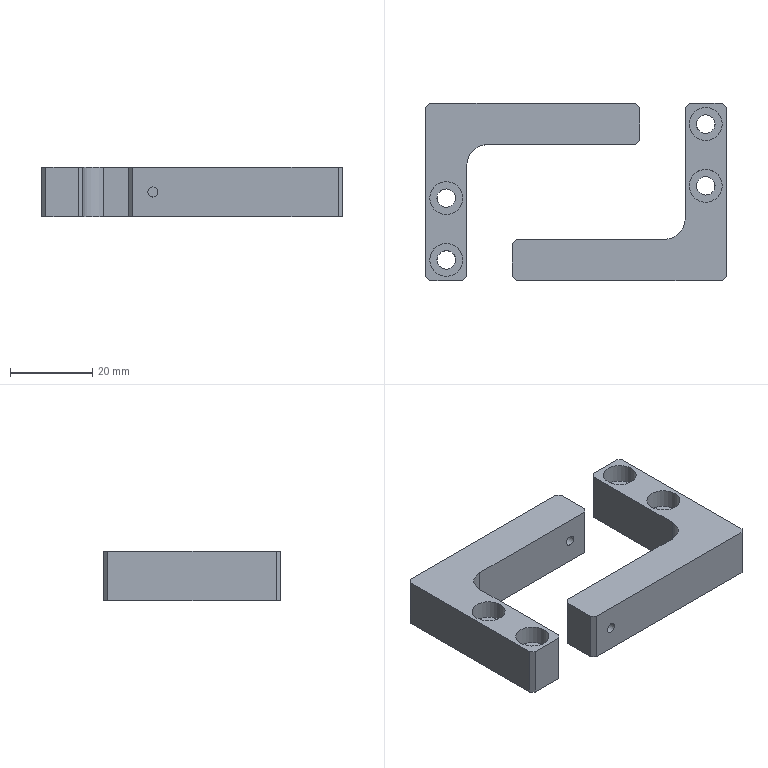Part | NX | 2 solids | 42 faces | box 73 x 43 x 12 mm | volume 18978 mm3 | plane 30 | cylinder 12 | commonest cylinder face diameters 4.5 x4 8 x4 2.459 x2 10 x2
STEP:
#1=CARTESIAN_POINT('',(-25.,-21.5,0.));
#2=VERTEX_POINT('',#1);
#3=CARTESIAN_POINT('',(-17.,-21.5,0.));
#4=VERTEX_POINT('',#3);
#5=CARTESIAN_POINT('',(-26.,-21.5,0.));
#6=DIRECTION('',(1.,0.,0.));
#7=VECTOR('',#6,1000.);
#8=LINE('',#5,#7);
#9=EDGE_CURVE('',#2,#4,#8,.T.);
#10=ORIENTED_EDGE('',*,*,#9,.F.);
#11=CARTESIAN_POINT('',(-25.,-21.5,-12.));
#12=VERTEX_POINT('',#11);
#13=CARTESIAN_POINT('',(-25.,-21.5,0.));
#14=DIRECTION('',(0.,0.,-1.));
#15=VECTOR('',#14,1000.);
#16=LINE('',#13,#15);
#17=EDGE_CURVE('',#2,#12,#16,.T.);
#18=ORIENTED_EDGE('',*,*,#17,.T.);
#19=CARTESIAN_POINT('',(-17.,-21.5,-12.));
#20=VERTEX_POINT('',#19);
#21=CARTESIAN_POINT('',(-26.,-21.5,-12.));
#22=DIRECTION('',(1.,0.,0.));
#23=VECTOR('',#22,1000.);
#24=LINE('',#21,#23);
#25=EDGE_CURVE('',#12,#20,#24,.T.);
#26=ORIENTED_EDGE('',*,*,#25,.T.);
#27=CARTESIAN_POINT('',(-17.,-21.5,0.));
#28=DIRECTION('',(0.,0.,1.));
#29=VECTOR('',#28,1000.);
#30=LINE('',#27,#29);
#31=EDGE_CURVE('',#20,#4,#30,.T.);
#32=ORIENTED_EDGE('',*,*,#31,.T.);
#33=EDGE_LOOP('',(#10,#18,#26,#32));
#34=FACE_BOUND('',#33,.T.);
#35=CARTESIAN_POINT('',(-26.,-21.5,0.));
#36=DIRECTION('',(0.,1.,0.));
#37=DIRECTION('',(0.,0.,1.));
#38=AXIS2_PLACEMENT_3D('',#35,#36,#37);
#39=PLANE('',#38);
#40=ADVANCED_FACE('',(#34),#39,.F.);
#41=CARTESIAN_POINT('',(-21.,0.75,-12.));
#42=VERTEX_POINT('',#41);
#43=CARTESIAN_POINT('',(-21.,-1.5,-12.));
#44=DIRECTION('',(0.,0.,1.));
#45=DIRECTION('',(0.,1.,0.));
#46=AXIS2_PLACEMENT_3D('',#43,#44,#45);
#47=CIRCLE('',#46,2.25);
#48=EDGE_CURVE('',#42,#42,#47,.T.);
#49=ORIENTED_EDGE('',*,*,#48,.T.);
#50=EDGE_LOOP('',(#49));
#51=FACE_BOUND('',#50,.T.);
#52=CARTESIAN_POINT('',(-21.,-14.25,-12.));
#53=VERTEX_POINT('',#52);
#54=CARTESIAN_POINT('',(-21.,-16.5,-12.));
#55=DIRECTION('',(0.,0.,1.));
#56=DIRECTION('',(0.,1.,0.));
#57=AXIS2_PLACEMENT_3D('',#54,#55,#56);
#58=CIRCLE('',#57,2.25);
#59=EDGE_CURVE('',#53,#53,#58,.T.);
#60=ORIENTED_EDGE('',*,*,#59,.T.);
#61=EDGE_LOOP('',(#60));
#62=FACE_BOUND('',#61,.T.);
#63=CARTESIAN_POINT('',(26.,12.5,-12.));
#64=VERTEX_POINT('',#63);
#65=CARTESIAN_POINT('',(26.,20.5,-12.));
#66=VERTEX_POINT('',#65);
#67=CARTESIAN_POINT('',(26.,-21.5,-12.));
#68=DIRECTION('',(0.,1.,0.));
#69=VECTOR('',#68,1000.);
#70=LINE('',#67,#69);
#71=EDGE_CURVE('',#64,#66,#70,.T.);
#72=ORIENTED_EDGE('',*,*,#71,.F.);
#73=CARTESIAN_POINT('',(25.,11.5,-12.));
#74=VERTEX_POINT('',#73);
#75=CARTESIAN_POINT('',(26.,12.5,-12.));
#76=DIRECTION('',(-0.7071,-0.7071,0.));
#77=VECTOR('',#76,1000.);
#78=LINE('',#75,#77);
#79=EDGE_CURVE('',#64,#74,#78,.T.);
#80=ORIENTED_EDGE('',*,*,#79,.T.);
#81=CARTESIAN_POINT('',(-11.,11.5,-12.));
#82=VERTEX_POINT('',#81);
#83=CARTESIAN_POINT('',(-16.,11.5,-12.));
#84=DIRECTION('',(1.,0.,0.));
#85=VECTOR('',#84,1000.);
#86=LINE('',#83,#85);
#87=EDGE_CURVE('',#82,#74,#86,.T.);
#88=ORIENTED_EDGE('',*,*,#87,.F.);
#89=CARTESIAN_POINT('',(-16.,6.5,-12.));
#90=VERTEX_POINT('',#89);
#91=CARTESIAN_POINT('',(-11.,6.5,-12.));
#92=DIRECTION('',(0.,0.,1.));
#93=DIRECTION('',(0.,1.,0.));
#94=AXIS2_PLACEMENT_3D('',#91,#92,#93);
#95=CIRCLE('',#94,5.);
#96=EDGE_CURVE('',#82,#90,#95,.T.);
#97=ORIENTED_EDGE('',*,*,#96,.T.);
#98=CARTESIAN_POINT('',(-16.,-20.5,-12.));
#99=VERTEX_POINT('',#98);
#100=CARTESIAN_POINT('',(-16.,-21.5,-12.));
#101=DIRECTION('',(0.,1.,0.));
#102=VECTOR('',#101,1000.);
#103=LINE('',#100,#102);
#104=EDGE_CURVE('',#99,#90,#103,.T.);
#105=ORIENTED_EDGE('',*,*,#104,.F.);
#106=CARTESIAN_POINT('',(-16.,-20.5,-12.));
#107=DIRECTION('',(-0.7071,-0.7071,0.));
#108=VECTOR('',#107,1000.);
#109=LINE('',#106,#108);
#110=EDGE_CURVE('',#99,#20,#109,.T.);
#111=ORIENTED_EDGE('',*,*,#110,.T.);
#112=ORIENTED_EDGE('',*,*,#25,.F.);
#113=CARTESIAN_POINT('',(-26.,-20.5,-12.));
#114=VERTEX_POINT('',#113);
#115=CARTESIAN_POINT('',(-25.,-21.5,-12.));
#116=DIRECTION('',(-0.7071,0.7071,0.));
#117=VECTOR('',#116,1000.);
#118=LINE('',#115,#117);
#119=EDGE_CURVE('',#12,#114,#118,.T.);
#120=ORIENTED_EDGE('',*,*,#119,.T.);
#121=CARTESIAN_POINT('',(-26.,20.5,-12.));
#122=VERTEX_POINT('',#121);
#123=CARTESIAN_POINT('',(-26.,21.5,-12.));
#124=DIRECTION('',(0.,-1.,0.));
#125=VECTOR('',#124,1000.);
#126=LINE('',#123,#125);
#127=EDGE_CURVE('',#122,#114,#126,.T.);
#128=ORIENTED_EDGE('',*,*,#127,.F.);
#129=CARTESIAN_POINT('',(-25.,21.5,-12.));
#130=VERTEX_POINT('',#129);
#131=CARTESIAN_POINT('',(-26.,20.5,-12.));
#132=DIRECTION('',(0.7071,0.7071,0.));
#133=VECTOR('',#132,1000.);
#134=LINE('',#131,#133);
#135=EDGE_CURVE('',#122,#130,#134,.T.);
#136=ORIENTED_EDGE('',*,*,#135,.T.);
#137=CARTESIAN_POINT('',(25.,21.5,-12.));
#138=VERTEX_POINT('',#137);
#139=CARTESIAN_POINT('',(26.,21.5,-12.));
#140=DIRECTION('',(-1.,0.,0.));
#141=VECTOR('',#140,1000.);
#142=LINE('',#139,#141);
#143=EDGE_CURVE('',#138,#130,#142,.T.);
#144=ORIENTED_EDGE('',*,*,#143,.F.);
#145=CARTESIAN_POINT('',(25.,21.5,-12.));
#146=DIRECTION('',(0.7071,-0.7071,0.));
#147=VECTOR('',#146,1000.);
#148=LINE('',#145,#147);
#149=EDGE_CURVE('',#138,#66,#148,.T.);
#150=ORIENTED_EDGE('',*,*,#149,.T.);
#151=EDGE_LOOP('',(#72,#80,#88,#97,#105,#111,#112,#120,#128,#136,#144,#150));
#152=FACE_BOUND('',#151,.T.);
#153=CARTESIAN_POINT('',(0.,0.,-12.));
#154=DIRECTION('',(0.,0.,1.));
#155=DIRECTION('',(0.,-1.,0.));
#156=AXIS2_PLACEMENT_3D('',#153,#154,#155);
#157=PLANE('',#156);
#158=ADVANCED_FACE('',(#51,#62,#152),#157,.F.);
#159=CARTESIAN_POINT('',(20.,21.5,-4.771));
#160=VERTEX_POINT('',#159);
#161=CARTESIAN_POINT('',(20.,21.5,-6.));
#162=DIRECTION('',(0.,-1.,0.));
#163=DIRECTION('',(0.,0.,1.));
#164=AXIS2_PLACEMENT_3D('',#161,#162,#163);
#165=CIRCLE('',#164,1.23);
#166=EDGE_CURVE('',#160,#160,#165,.T.);
#167=ORIENTED_EDGE('',*,*,#166,.T.);
#168=EDGE_LOOP('',(#167));
#169=FACE_BOUND('',#168,.T.);
#170=CARTESIAN_POINT('',(25.,21.5,0.));
#171=VERTEX_POINT('',#170);
#172=CARTESIAN_POINT('',(-25.,21.5,0.));
#173=VERTEX_POINT('',#172);
#174=CARTESIAN_POINT('',(26.,21.5,0.));
#175=DIRECTION('',(-1.,0.,0.));
#176=VECTOR('',#175,1000.);
#177=LINE('',#174,#176);
#178=EDGE_CURVE('',#171,#173,#177,.T.);
#179=ORIENTED_EDGE('',*,*,#178,.F.);
#180=CARTESIAN_POINT('',(25.,21.5,0.));
#181=DIRECTION('',(0.,0.,-1.));
#182=VECTOR('',#181,1000.);
#183=LINE('',#180,#182);
#184=EDGE_CURVE('',#171,#138,#183,.T.);
#185=ORIENTED_EDGE('',*,*,#184,.T.);
#186=ORIENTED_EDGE('',*,*,#143,.T.);
#187=CARTESIAN_POINT('',(-25.,21.5,0.));
#188=DIRECTION('',(0.,0.,1.));
#189=VECTOR('',#188,1000.);
#190=LINE('',#187,#189);
#191=EDGE_CURVE('',#130,#173,#190,.T.);
#192=ORIENTED_EDGE('',*,*,#191,.T.);
#193=EDGE_LOOP('',(#179,#185,#186,#192));
#194=FACE_BOUND('',#193,.T.);
#195=CARTESIAN_POINT('',(26.,21.5,0.));
#196=DIRECTION('',(0.,-1.,0.));
#197=DIRECTION('',(0.,0.,-1.));
#198=AXIS2_PLACEMENT_3D('',#195,#196,#197);
#199=PLANE('',#198);
#200=ADVANCED_FACE('',(#169,#194),#199,.F.);
#201=CARTESIAN_POINT('',(-26.,20.5,0.));
#202=VERTEX_POINT('',#201);
#203=CARTESIAN_POINT('',(-26.,-20.5,0.));
#204=VERTEX_POINT('',#203);
#205=CARTESIAN_POINT('',(-26.,21.5,0.));
#206=DIRECTION('',(0.,-1.,0.));
#207=VECTOR('',#206,1000.);
#208=LINE('',#205,#207);
#209=EDGE_CURVE('',#202,#204,#208,.T.);
#210=ORIENTED_EDGE('',*,*,#209,.F.);
#211=CARTESIAN_POINT('',(-26.,20.5,0.));
#212=DIRECTION('',(0.,0.,-1.));
#213=VECTOR('',#212,1000.);
#214=LINE('',#211,#213);
#215=EDGE_CURVE('',#202,#122,#214,.T.);
#216=ORIENTED_EDGE('',*,*,#215,.T.);
#217=ORIENTED_EDGE('',*,*,#127,.T.);
#218=CARTESIAN_POINT('',(-26.,-20.5,0.));
#219=DIRECTION('',(0.,0.,1.));
#220=VECTOR('',#219,1000.);
#221=LINE('',#218,#220);
#222=EDGE_CURVE('',#114,#204,#221,.T.);
#223=ORIENTED_EDGE('',*,*,#222,.T.);
#224=EDGE_LOOP('',(#210,#216,#217,#223));
#225=FACE_BOUND('',#224,.T.);
#226=CARTESIAN_POINT('',(-26.,21.5,0.));
#227=DIRECTION('',(1.,0.,0.));
#228=DIRECTION('',(0.,0.,-1.));
#229=AXIS2_PLACEMENT_3D('',#226,#227,#228);
#230=PLANE('',#229);
#231=ADVANCED_FACE('',(#225),#230,.F.);
#232=CARTESIAN_POINT('',(26.,12.5,0.));
#233=VERTEX_POINT('',#232);
#234=CARTESIAN_POINT('',(26.,20.5,0.));
#235=VERTEX_POINT('',#234);
#236=CARTESIAN_POINT('',(26.,-21.5,0.));
#237=DIRECTION('',(0.,1.,0.));
#238=VECTOR('',#237,1000.);
#239=LINE('',#236,#238);
#240=EDGE_CURVE('',#233,#235,#239,.T.);
#241=ORIENTED_EDGE('',*,*,#240,.F.);
#242=CARTESIAN_POINT('',(26.,12.5,0.));
#243=DIRECTION('',(0.,0.,-1.));
#244=VECTOR('',#243,1000.);
#245=LINE('',#242,#244);
#246=EDGE_CURVE('',#233,#64,#245,.T.);
#247=ORIENTED_EDGE('',*,*,#246,.T.);
#248=ORIENTED_EDGE('',*,*,#71,.T.);
#249=CARTESIAN_POINT('',(26.,20.5,0.));
#250=DIRECTION('',(0.,0.,1.));
#251=VECTOR('',#250,1000.);
#252=LINE('',#249,#251);
#253=EDGE_CURVE('',#66,#235,#252,.T.);
#254=ORIENTED_EDGE('',*,*,#253,.T.);
#255=EDGE_LOOP('',(#241,#247,#248,#254));
#256=FACE_BOUND('',#255,.T.);
#257=CARTESIAN_POINT('',(26.,-21.5,0.));
#258=DIRECTION('',(-1.,0.,0.));
#259=DIRECTION('',(0.,0.,1.));
#260=AXIS2_PLACEMENT_3D('',#257,#258,#259);
#261=PLANE('',#260);
#262=ADVANCED_FACE('',(#256),#261,.F.);
#263=CARTESIAN_POINT('',(-25.,-1.5,0.));
#264=VERTEX_POINT('',#263);
#265=CARTESIAN_POINT('',(-21.,-1.5,0.));
#266=DIRECTION('',(0.,0.,-1.));
#267=DIRECTION('',(-1.,0.,0.));
#268=AXIS2_PLACEMENT_3D('',#265,#266,#267);
#269=CIRCLE('',#268,4.);
#270=EDGE_CURVE('',#264,#264,#269,.T.);
#271=ORIENTED_EDGE('',*,*,#270,.T.);
#272=EDGE_LOOP('',(#271));
#273=FACE_BOUND('',#272,.T.);
#274=CARTESIAN_POINT('',(-25.,-16.5,0.));
#275=VERTEX_POINT('',#274);
#276=CARTESIAN_POINT('',(-21.,-16.5,0.));
#277=DIRECTION('',(0.,0.,-1.));
#278=DIRECTION('',(-1.,0.,0.));
#279=AXIS2_PLACEMENT_3D('',#276,#277,#278);
#280=CIRCLE('',#279,4.);
#281=EDGE_CURVE('',#275,#275,#280,.T.);
#282=ORIENTED_EDGE('',*,*,#281,.T.);
#283=EDGE_LOOP('',(#282));
#284=FACE_BOUND('',#283,.T.);
#285=CARTESIAN_POINT('',(25.,11.5,0.));
#286=VERTEX_POINT('',#285);
#287=CARTESIAN_POINT('',(-11.,11.5,0.));
#288=VERTEX_POINT('',#287);
#289=CARTESIAN_POINT('',(0.,11.5,0.));
#290=DIRECTION('',(-1.,0.,0.));
#291=VECTOR('',#290,1000.);
#292=LINE('',#289,#291);
#293=EDGE_CURVE('',#286,#288,#292,.T.);
#294=ORIENTED_EDGE('',*,*,#293,.F.);
#295=CARTESIAN_POINT('',(6.75,-6.75,0.));
#296=DIRECTION('',(0.7071,0.7071,0.));
#297=VECTOR('',#296,1000.);
#298=LINE('',#295,#297);
#299=EDGE_CURVE('',#286,#233,#298,.T.);
#300=ORIENTED_EDGE('',*,*,#299,.T.);
#301=ORIENTED_EDGE('',*,*,#240,.T.);
#302=CARTESIAN_POINT('',(23.25,23.25,0.));
#303=DIRECTION('',(-0.7071,0.7071,0.));
#304=VECTOR('',#303,1000.);
#305=LINE('',#302,#304);
#306=EDGE_CURVE('',#235,#171,#305,.T.);
#307=ORIENTED_EDGE('',*,*,#306,.T.);
#308=ORIENTED_EDGE('',*,*,#178,.T.);
#309=CARTESIAN_POINT('',(-23.25,23.25,0.));
#310=DIRECTION('',(-0.7071,-0.7071,0.));
#311=VECTOR('',#310,1000.);
#312=LINE('',#309,#311);
#313=EDGE_CURVE('',#173,#202,#312,.T.);
#314=ORIENTED_EDGE('',*,*,#313,.T.);
#315=ORIENTED_EDGE('',*,*,#209,.T.);
#316=CARTESIAN_POINT('',(-23.25,-23.25,0.));
#317=DIRECTION('',(0.7071,-0.7071,0.));
#318=VECTOR('',#317,1000.);
#319=LINE('',#316,#318);
#320=EDGE_CURVE('',#204,#2,#319,.T.);
#321=ORIENTED_EDGE('',*,*,#320,.T.);
#322=ORIENTED_EDGE('',*,*,#9,.T.);
#323=CARTESIAN_POINT('',(-16.,-20.5,0.));
#324=VERTEX_POINT('',#323);
#325=CARTESIAN_POINT('',(2.25,-2.25,0.));
#326=DIRECTION('',(0.7071,0.7071,0.));
#327=VECTOR('',#326,1000.);
#328=LINE('',#325,#327);
#329=EDGE_CURVE('',#4,#324,#328,.T.);
#330=ORIENTED_EDGE('',*,*,#329,.T.);
#331=CARTESIAN_POINT('',(-16.,6.5,0.));
#332=VERTEX_POINT('',#331);
#333=CARTESIAN_POINT('',(-16.,0.,0.));
#334=DIRECTION('',(0.,-1.,0.));
#335=VECTOR('',#334,1000.);
#336=LINE('',#333,#335);
#337=EDGE_CURVE('',#332,#324,#336,.T.);
#338=ORIENTED_EDGE('',*,*,#337,.F.);
#339=CARTESIAN_POINT('',(-11.,6.5,0.));
#340=DIRECTION('',(0.,0.,-1.));
#341=DIRECTION('',(0.,1.,0.));
#342=AXIS2_PLACEMENT_3D('',#339,#340,#341);
#343=CIRCLE('',#342,5.);
#344=EDGE_CURVE('',#332,#288,#343,.T.);
#345=ORIENTED_EDGE('',*,*,#344,.T.);
#346=EDGE_LOOP('',(#294,#300,#301,#307,#308,#314,#315,#321,#322,#330,#338,#345));
#347=FACE_BOUND('',#346,.T.);
#348=CARTESIAN_POINT('',(0.,0.,0.));
#349=DIRECTION('',(0.,0.,1.));
#350=DIRECTION('',(0.,-1.,0.));
#351=AXIS2_PLACEMENT_3D('',#348,#349,#350);
#352=PLANE('',#351);
#353=ADVANCED_FACE('',(#273,#284,#347),#352,.T.);
#354=ORIENTED_EDGE('',*,*,#104,.T.);
#355=CARTESIAN_POINT('',(-16.,6.5,0.));
#356=DIRECTION('',(0.,0.,1.));
#357=VECTOR('',#356,1000.);
#358=LINE('',#355,#357);
#359=EDGE_CURVE('',#90,#332,#358,.T.);
#360=ORIENTED_EDGE('',*,*,#359,.T.);
#361=ORIENTED_EDGE('',*,*,#337,.T.);
#362=CARTESIAN_POINT('',(-16.,-20.5,91.5));
#363=DIRECTION('',(0.,0.,-1.));
#364=VECTOR('',#363,1000.);
#365=LINE('',#362,#364);
#366=EDGE_CURVE('',#324,#99,#365,.T.);
#367=ORIENTED_EDGE('',*,*,#366,.T.);
#368=EDGE_LOOP('',(#354,#360,#361,#367));
#369=FACE_BOUND('',#368,.T.);
#370=CARTESIAN_POINT('',(-16.,-21.5,91.5));
#371=DIRECTION('',(-1.,0.,0.));
#372=DIRECTION('',(0.,0.,1.));
#373=AXIS2_PLACEMENT_3D('',#370,#371,#372);
#374=PLANE('',#373);
#375=ADVANCED_FACE('',(#369),#374,.F.);
#376=CARTESIAN_POINT('',(18.77,11.5,-6.));
#377=VERTEX_POINT('',#376);
#378=CARTESIAN_POINT('',(20.,11.5,-6.));
#379=DIRECTION('',(0.,1.,0.));
#380=DIRECTION('',(-1.,0.,0.));
#381=AXIS2_PLACEMENT_3D('',#378,#379,#380);
#382=CIRCLE('',#381,1.23);
#383=EDGE_CURVE('',#377,#377,#382,.T.);
#384=ORIENTED_EDGE('',*,*,#383,.T.);
#385=EDGE_LOOP('',(#384));
#386=FACE_BOUND('',#385,.T.);
#387=ORIENTED_EDGE('',*,*,#293,.T.);
#388=CARTESIAN_POINT('',(-11.,11.5,-12.));
#389=DIRECTION('',(0.,0.,-1.));
#390=VECTOR('',#389,1000.);
#391=LINE('',#388,#390);
#392=EDGE_CURVE('',#288,#82,#391,.T.);
#393=ORIENTED_EDGE('',*,*,#392,.T.);
#394=ORIENTED_EDGE('',*,*,#87,.T.);
#395=CARTESIAN_POINT('',(25.,11.5,91.5));
#396=DIRECTION('',(0.,0.,1.));
#397=VECTOR('',#396,1000.);
#398=LINE('',#395,#397);
#399=EDGE_CURVE('',#74,#286,#398,.T.);
#400=ORIENTED_EDGE('',*,*,#399,.T.);
#401=EDGE_LOOP('',(#387,#393,#394,#400));
#402=FACE_BOUND('',#401,.T.);
#403=CARTESIAN_POINT('',(-16.,11.5,91.5));
#404=DIRECTION('',(0.,1.,0.));
#405=DIRECTION('',(-1.,0.,0.));
#406=AXIS2_PLACEMENT_3D('',#403,#404,#405);
#407=PLANE('',#406);
#408=ADVANCED_FACE('',(#386,#402),#407,.F.);
#409=ORIENTED_EDGE('',*,*,#299,.F.);
#410=ORIENTED_EDGE('',*,*,#399,.F.);
#411=ORIENTED_EDGE('',*,*,#79,.F.);
#412=ORIENTED_EDGE('',*,*,#246,.F.);
#413=EDGE_LOOP('',(#409,#410,#411,#412));
#414=FACE_BOUND('',#413,.T.);
#415=CARTESIAN_POINT('',(26.,12.5,0.));
#416=DIRECTION('',(-0.7071,0.7071,0.));
#417=DIRECTION('',(0.,0.,1.));
#418=AXIS2_PLACEMENT_3D('',#415,#416,#417);
#419=PLANE('',#418);
#420=ADVANCED_FACE('',(#414),#419,.F.);
#421=ORIENTED_EDGE('',*,*,#306,.F.);
#422=ORIENTED_EDGE('',*,*,#253,.F.);
#423=ORIENTED_EDGE('',*,*,#149,.F.);
#424=ORIENTED_EDGE('',*,*,#184,.F.);
#425=EDGE_LOOP('',(#421,#422,#423,#424));
#426=FACE_BOUND('',#425,.T.);
#427=CARTESIAN_POINT('',(25.,21.5,0.));
#428=DIRECTION('',(-0.7071,-0.7071,0.));
#429=DIRECTION('',(0.,0.,1.));
#430=AXIS2_PLACEMENT_3D('',#427,#428,#429);
#431=PLANE('',#430);
#432=ADVANCED_FACE('',(#426),#431,.F.);
#433=ORIENTED_EDGE('',*,*,#313,.F.);
#434=ORIENTED_EDGE('',*,*,#191,.F.);
#435=ORIENTED_EDGE('',*,*,#135,.F.);
#436=ORIENTED_EDGE('',*,*,#215,.F.);
#437=EDGE_LOOP('',(#433,#434,#435,#436));
#438=FACE_BOUND('',#437,.T.);
#439=CARTESIAN_POINT('',(-26.,20.5,0.));
#440=DIRECTION('',(0.7071,-0.7071,0.));
#441=DIRECTION('',(0.,0.,1.));
#442=AXIS2_PLACEMENT_3D('',#439,#440,#441);
#443=PLANE('',#442);
#444=ADVANCED_FACE('',(#438),#443,.F.);
#445=ORIENTED_EDGE('',*,*,#320,.F.);
#446=ORIENTED_EDGE('',*,*,#222,.F.);
#447=ORIENTED_EDGE('',*,*,#119,.F.);
#448=ORIENTED_EDGE('',*,*,#17,.F.);
#449=EDGE_LOOP('',(#445,#446,#447,#448));
#450=FACE_BOUND('',#449,.T.);
#451=CARTESIAN_POINT('',(-25.,-21.5,0.));
#452=DIRECTION('',(0.7071,0.7071,0.));
#453=DIRECTION('',(0.,0.,1.));
#454=AXIS2_PLACEMENT_3D('',#451,#452,#453);
#455=PLANE('',#454);
#456=ADVANCED_FACE('',(#450),#455,.F.);
#457=ORIENTED_EDGE('',*,*,#329,.F.);
#458=ORIENTED_EDGE('',*,*,#31,.F.);
#459=ORIENTED_EDGE('',*,*,#110,.F.);
#460=ORIENTED_EDGE('',*,*,#366,.F.);
#461=EDGE_LOOP('',(#457,#458,#459,#460));
#462=FACE_BOUND('',#461,.T.);
#463=CARTESIAN_POINT('',(-16.,-20.5,91.5));
#464=DIRECTION('',(-0.7071,0.7071,0.));
#465=DIRECTION('',(0.,0.,1.));
#466=AXIS2_PLACEMENT_3D('',#463,#464,#465);
#467=PLANE('',#466);
#468=ADVANCED_FACE('',(#462),#467,.F.);
#469=ORIENTED_EDGE('',*,*,#344,.F.);
#470=ORIENTED_EDGE('',*,*,#359,.F.);
#471=ORIENTED_EDGE('',*,*,#96,.F.);
#472=ORIENTED_EDGE('',*,*,#392,.F.);
#473=EDGE_LOOP('',(#469,#470,#471,#472));
#474=FACE_BOUND('',#473,.T.);
#475=CARTESIAN_POINT('',(-11.,6.5,91.5));
#476=DIRECTION('',(0.,0.,1.));
#477=DIRECTION('',(0.,-1.,0.));
#478=AXIS2_PLACEMENT_3D('',#475,#476,#477);
#479=CYLINDRICAL_SURFACE('',#478,5.);
#480=ADVANCED_FACE('',(#474),#479,.F.);
#481=ORIENTED_EDGE('',*,*,#383,.F.);
#482=EDGE_LOOP('',(#481));
#483=FACE_BOUND('',#482,.T.);
#484=ORIENTED_EDGE('',*,*,#166,.F.);
#485=EDGE_LOOP('',(#484));
#486=FACE_BOUND('',#485,.T.);
#487=CARTESIAN_POINT('',(20.,11.5,-6.));
#488=DIRECTION('',(0.,1.,0.));
#489=DIRECTION('',(1.,0.,0.));
#490=AXIS2_PLACEMENT_3D('',#487,#488,#489);
#491=CYLINDRICAL_SURFACE('',#490,1.23);
#492=ADVANCED_FACE('',(#483,#486),#491,.F.);
#493=CARTESIAN_POINT('',(-23.25,-16.5,-4.6));
#494=VERTEX_POINT('',#493);
#495=CARTESIAN_POINT('',(-21.,-16.5,-4.6));
#496=DIRECTION('',(0.,0.,-1.));
#497=DIRECTION('',(-1.,0.,0.));
#498=AXIS2_PLACEMENT_3D('',#495,#496,#497);
#499=CIRCLE('',#498,2.25);
#500=EDGE_CURVE('',#494,#494,#499,.T.);
#501=ORIENTED_EDGE('',*,*,#500,.F.);
#502=EDGE_LOOP('',(#501));
#503=FACE_BOUND('',#502,.T.);
#504=ORIENTED_EDGE('',*,*,#59,.F.);
#505=EDGE_LOOP('',(#504));
#506=FACE_BOUND('',#505,.T.);
#507=CARTESIAN_POINT('',(-21.,-16.5,-4.6));
#508=DIRECTION('',(0.,0.,-1.));
#509=DIRECTION('',(1.,0.,0.));
#510=AXIS2_PLACEMENT_3D('',#507,#508,#509);
#511=CYLINDRICAL_SURFACE('',#510,2.25);
#512=ADVANCED_FACE('',(#503,#506),#511,.F.);
#513=ORIENTED_EDGE('',*,*,#500,.T.);
#514=EDGE_LOOP('',(#513));
#515=FACE_BOUND('',#514,.T.);
#516=CARTESIAN_POINT('',(-25.,-16.5,-4.6));
#517=VERTEX_POINT('',#516);
#518=CARTESIAN_POINT('',(-21.,-16.5,-4.6));
#519=DIRECTION('',(0.,0.,1.));
#520=DIRECTION('',(-1.,0.,0.));
#521=AXIS2_PLACEMENT_3D('',#518,#519,#520);
#522=CIRCLE('',#521,4.);
#523=EDGE_CURVE('',#517,#517,#522,.T.);
#524=ORIENTED_EDGE('',*,*,#523,.T.);
#525=EDGE_LOOP('',(#524));
#526=FACE_BOUND('',#525,.T.);
#527=CARTESIAN_POINT('',(-21.,-16.5,-4.6));
#528=DIRECTION('',(0.,0.,-1.));
#529=DIRECTION('',(0.,1.,0.));
#530=AXIS2_PLACEMENT_3D('',#527,#528,#529);
#531=PLANE('',#530);
#532=ADVANCED_FACE('',(#515,#526),#531,.F.);
#533=ORIENTED_EDGE('',*,*,#523,.F.);
#534=EDGE_LOOP('',(#533));
#535=FACE_BOUND('',#534,.T.);
#536=ORIENTED_EDGE('',*,*,#281,.F.);
#537=EDGE_LOOP('',(#536));
#538=FACE_BOUND('',#537,.T.);
#539=CARTESIAN_POINT('',(-21.,-16.5,0.));
#540=DIRECTION('',(0.,0.,-1.));
#541=DIRECTION('',(1.,0.,0.));
#542=AXIS2_PLACEMENT_3D('',#539,#540,#541);
#543=CYLINDRICAL_SURFACE('',#542,4.);
#544=ADVANCED_FACE('',(#535,#538),#543,.F.);
#545=CARTESIAN_POINT('',(-23.25,-1.5,-4.6));
#546=VERTEX_POINT('',#545);
#547=CARTESIAN_POINT('',(-21.,-1.5,-4.6));
#548=DIRECTION('',(0.,0.,-1.));
#549=DIRECTION('',(-1.,0.,0.));
#550=AXIS2_PLACEMENT_3D('',#547,#548,#549);
#551=CIRCLE('',#550,2.25);
#552=EDGE_CURVE('',#546,#546,#551,.T.);
#553=ORIENTED_EDGE('',*,*,#552,.F.);
#554=EDGE_LOOP('',(#553));
#555=FACE_BOUND('',#554,.T.);
#556=ORIENTED_EDGE('',*,*,#48,.F.);
#557=EDGE_LOOP('',(#556));
#558=FACE_BOUND('',#557,.T.);
#559=CARTESIAN_POINT('',(-21.,-1.5,-4.6));
#560=DIRECTION('',(0.,0.,-1.));
#561=DIRECTION('',(1.,0.,0.));
#562=AXIS2_PLACEMENT_3D('',#559,#560,#561);
#563=CYLINDRICAL_SURFACE('',#562,2.25);
#564=ADVANCED_FACE('',(#555,#558),#563,.F.);
#565=ORIENTED_EDGE('',*,*,#552,.T.);
#566=EDGE_LOOP('',(#565));
#567=FACE_BOUND('',#566,.T.);
#568=CARTESIAN_POINT('',(-25.,-1.5,-4.6));
#569=VERTEX_POINT('',#568);
#570=CARTESIAN_POINT('',(-21.,-1.5,-4.6));
#571=DIRECTION('',(0.,0.,1.));
#572=DIRECTION('',(-1.,0.,0.));
#573=AXIS2_PLACEMENT_3D('',#570,#571,#572);
#574=CIRCLE('',#573,4.);
#575=EDGE_CURVE('',#569,#569,#574,.T.);
#576=ORIENTED_EDGE('',*,*,#575,.T.);
#577=EDGE_LOOP('',(#576));
#578=FACE_BOUND('',#577,.T.);
#579=CARTESIAN_POINT('',(-21.,-1.5,-4.6));
#580=DIRECTION('',(0.,0.,-1.));
#581=DIRECTION('',(0.,1.,0.));
#582=AXIS2_PLACEMENT_3D('',#579,#580,#581);
#583=PLANE('',#582);
#584=ADVANCED_FACE('',(#567,#578),#583,.F.);
#585=ORIENTED_EDGE('',*,*,#575,.F.);
#586=EDGE_LOOP('',(#585));
#587=FACE_BOUND('',#586,.T.);
#588=ORIENTED_EDGE('',*,*,#270,.F.);
#589=EDGE_LOOP('',(#588));
#590=FACE_BOUND('',#589,.T.);
#591=CARTESIAN_POINT('',(-21.,-1.5,0.));
#592=DIRECTION('',(0.,0.,-1.));
#593=DIRECTION('',(1.,0.,0.));
#594=AXIS2_PLACEMENT_3D('',#591,#592,#593);
#595=CYLINDRICAL_SURFACE('',#594,4.);
#596=ADVANCED_FACE('',(#587,#590),#595,.F.);
#597=CLOSED_SHELL('',(#40,#158,#200,#231,#262,#353,#375,#408,#420,#432,#444,#456,#468,#480,#492,#512,#532,#544,#564,#584,#596));
#598=MANIFOLD_SOLID_BREP('',#597);
#599=CARTESIAN_POINT('',(46.,21.5,0.));
#600=VERTEX_POINT('',#599);
#601=CARTESIAN_POINT('',(38.,21.5,0.));
#602=VERTEX_POINT('',#601);
#603=CARTESIAN_POINT('',(47.,21.5,0.));
#604=DIRECTION('',(-1.,0.,0.));
#605=VECTOR('',#604,1000.);
#606=LINE('',#603,#605);
#607=EDGE_CURVE('',#600,#602,#606,.T.);
#608=ORIENTED_EDGE('',*,*,#607,.F.);
#609=CARTESIAN_POINT('',(46.,21.5,-12.));
#610=VERTEX_POINT('',#609);
#611=CARTESIAN_POINT('',(46.,21.5,0.));
#612=DIRECTION('',(0.,0.,-1.));
#613=VECTOR('',#612,1000.);
#614=LINE('',#611,#613);
#615=EDGE_CURVE('',#600,#610,#614,.T.);
#616=ORIENTED_EDGE('',*,*,#615,.T.);
#617=CARTESIAN_POINT('',(38.,21.5,-12.));
#618=VERTEX_POINT('',#617);
#619=CARTESIAN_POINT('',(47.,21.5,-12.));
#620=DIRECTION('',(-1.,0.,0.));
#621=VECTOR('',#620,1000.);
#622=LINE('',#619,#621);
#623=EDGE_CURVE('',#610,#618,#622,.T.);
#624=ORIENTED_EDGE('',*,*,#623,.T.);
#625=CARTESIAN_POINT('',(38.,21.5,0.));
#626=DIRECTION('',(0.,0.,1.));
#627=VECTOR('',#626,1000.);
#628=LINE('',#625,#627);
#629=EDGE_CURVE('',#618,#602,#628,.T.);
#630=ORIENTED_EDGE('',*,*,#629,.T.);
#631=EDGE_LOOP('',(#608,#616,#624,#630));
#632=FACE_BOUND('',#631,.T.);
#633=CARTESIAN_POINT('',(47.,21.5,0.));
#634=DIRECTION('',(0.,-1.,0.));
#635=DIRECTION('',(0.,0.,1.));
#636=AXIS2_PLACEMENT_3D('',#633,#634,#635);
#637=PLANE('',#636);
#638=ADVANCED_FACE('',(#632),#637,.F.);
#639=CARTESIAN_POINT('',(42.,-0.75,-12.));
#640=VERTEX_POINT('',#639);
#641=CARTESIAN_POINT('',(42.,1.5,-12.));
#642=DIRECTION('',(0.,0.,1.));
#643=DIRECTION('',(0.,-1.,0.));
#644=AXIS2_PLACEMENT_3D('',#641,#642,#643);
#645=CIRCLE('',#644,2.25);
#646=EDGE_CURVE('',#640,#640,#645,.T.);
#647=ORIENTED_EDGE('',*,*,#646,.T.);
#648=EDGE_LOOP('',(#647));
#649=FACE_BOUND('',#648,.T.);
#650=CARTESIAN_POINT('',(42.,14.25,-12.));
#651=VERTEX_POINT('',#650);
#652=CARTESIAN_POINT('',(42.,16.5,-12.));
#653=DIRECTION('',(0.,0.,1.));
#654=DIRECTION('',(0.,-1.,0.));
#655=AXIS2_PLACEMENT_3D('',#652,#653,#654);
#656=CIRCLE('',#655,2.25);
#657=EDGE_CURVE('',#651,#651,#656,.T.);
#658=ORIENTED_EDGE('',*,*,#657,.T.);
#659=EDGE_LOOP('',(#658));
#660=FACE_BOUND('',#659,.T.);
#661=CARTESIAN_POINT('',(-5.,-12.5,-12.));
#662=VERTEX_POINT('',#661);
#663=CARTESIAN_POINT('',(-5.,-20.5,-12.));
#664=VERTEX_POINT('',#663);
#665=CARTESIAN_POINT('',(-5.,21.5,-12.));
#666=DIRECTION('',(0.,-1.,0.));
#667=VECTOR('',#666,1000.);
#668=LINE('',#665,#667);
#669=EDGE_CURVE('',#662,#664,#668,.T.);
#670=ORIENTED_EDGE('',*,*,#669,.F.);
#671=CARTESIAN_POINT('',(-4.,-11.5,-12.));
#672=VERTEX_POINT('',#671);
#673=CARTESIAN_POINT('',(-5.,-12.5,-12.));
#674=DIRECTION('',(0.7071,0.7071,0.));
#675=VECTOR('',#674,1000.);
#676=LINE('',#673,#675);
#677=EDGE_CURVE('',#662,#672,#676,.T.);
#678=ORIENTED_EDGE('',*,*,#677,.T.);
#679=CARTESIAN_POINT('',(32.,-11.5,-12.));
#680=VERTEX_POINT('',#679);
#681=CARTESIAN_POINT('',(37.,-11.5,-12.));
#682=DIRECTION('',(-1.,0.,0.));
#683=VECTOR('',#682,1000.);
#684=LINE('',#681,#683);
#685=EDGE_CURVE('',#680,#672,#684,.T.);
#686=ORIENTED_EDGE('',*,*,#685,.F.);
#687=CARTESIAN_POINT('',(37.,-6.5,-12.));
#688=VERTEX_POINT('',#687);
#689=CARTESIAN_POINT('',(32.,-6.5,-12.));
#690=DIRECTION('',(0.,0.,1.));
#691=DIRECTION('',(0.,-1.,0.));
#692=AXIS2_PLACEMENT_3D('',#689,#690,#691);
#693=CIRCLE('',#692,5.);
#694=EDGE_CURVE('',#680,#688,#693,.T.);
#695=ORIENTED_EDGE('',*,*,#694,.T.);
#696=CARTESIAN_POINT('',(37.,20.5,-12.));
#697=VERTEX_POINT('',#696);
#698=CARTESIAN_POINT('',(37.,21.5,-12.));
#699=DIRECTION('',(0.,-1.,0.));
#700=VECTOR('',#699,1000.);
#701=LINE('',#698,#700);
#702=EDGE_CURVE('',#697,#688,#701,.T.);
#703=ORIENTED_EDGE('',*,*,#702,.F.);
#704=CARTESIAN_POINT('',(37.,20.5,-12.));
#705=DIRECTION('',(0.7071,0.7071,0.));
#706=VECTOR('',#705,1000.);
#707=LINE('',#704,#706);
#708=EDGE_CURVE('',#697,#618,#707,.T.);
#709=ORIENTED_EDGE('',*,*,#708,.T.);
#710=ORIENTED_EDGE('',*,*,#623,.F.);
#711=CARTESIAN_POINT('',(47.,20.5,-12.));
#712=VERTEX_POINT('',#711);
#713=CARTESIAN_POINT('',(46.,21.5,-12.));
#714=DIRECTION('',(0.7071,-0.7071,0.));
#715=VECTOR('',#714,1000.);
#716=LINE('',#713,#715);
#717=EDGE_CURVE('',#610,#712,#716,.T.);
#718=ORIENTED_EDGE('',*,*,#717,.T.);
#719=CARTESIAN_POINT('',(47.,-20.5,-12.));
#720=VERTEX_POINT('',#719);
#721=CARTESIAN_POINT('',(47.,-21.5,-12.));
#722=DIRECTION('',(0.,1.,0.));
#723=VECTOR('',#722,1000.);
#724=LINE('',#721,#723);
#725=EDGE_CURVE('',#720,#712,#724,.T.);
#726=ORIENTED_EDGE('',*,*,#725,.F.);
#727=CARTESIAN_POINT('',(46.,-21.5,-12.));
#728=VERTEX_POINT('',#727);
#729=CARTESIAN_POINT('',(47.,-20.5,-12.));
#730=DIRECTION('',(-0.7071,-0.7071,0.));
#731=VECTOR('',#730,1000.);
#732=LINE('',#729,#731);
#733=EDGE_CURVE('',#720,#728,#732,.T.);
#734=ORIENTED_EDGE('',*,*,#733,.T.);
#735=CARTESIAN_POINT('',(-4.,-21.5,-12.));
#736=VERTEX_POINT('',#735);
#737=CARTESIAN_POINT('',(-5.,-21.5,-12.));
#738=DIRECTION('',(1.,0.,0.));
#739=VECTOR('',#738,1000.);
#740=LINE('',#737,#739);
#741=EDGE_CURVE('',#736,#728,#740,.T.);
#742=ORIENTED_EDGE('',*,*,#741,.F.);
#743=CARTESIAN_POINT('',(-4.,-21.5,-12.));
#744=DIRECTION('',(-0.7071,0.7071,0.));
#745=VECTOR('',#744,1000.);
#746=LINE('',#743,#745);
#747=EDGE_CURVE('',#736,#664,#746,.T.);
#748=ORIENTED_EDGE('',*,*,#747,.T.);
#749=EDGE_LOOP('',(#670,#678,#686,#695,#703,#709,#710,#718,#726,#734,#742,#748));
#750=FACE_BOUND('',#749,.T.);
#751=CARTESIAN_POINT('',(21.,0.,-12.));
#752=DIRECTION('',(0.,0.,1.));
#753=DIRECTION('',(0.,1.,0.));
#754=AXIS2_PLACEMENT_3D('',#751,#752,#753);
#755=PLANE('',#754);
#756=ADVANCED_FACE('',(#649,#660,#750),#755,.F.);
#757=CARTESIAN_POINT('',(1.,-21.5,-4.771));
#758=VERTEX_POINT('',#757);
#759=CARTESIAN_POINT('',(1.,-21.5,-6.));
#760=DIRECTION('',(0.,1.,0.));
#761=DIRECTION('',(0.,0.,1.));
#762=AXIS2_PLACEMENT_3D('',#759,#760,#761);
#763=CIRCLE('',#762,1.23);
#764=EDGE_CURVE('',#758,#758,#763,.T.);
#765=ORIENTED_EDGE('',*,*,#764,.T.);
#766=EDGE_LOOP('',(#765));
#767=FACE_BOUND('',#766,.T.);
#768=CARTESIAN_POINT('',(-4.,-21.5,0.));
#769=VERTEX_POINT('',#768);
#770=CARTESIAN_POINT('',(46.,-21.5,0.));
#771=VERTEX_POINT('',#770);
#772=CARTESIAN_POINT('',(-5.,-21.5,0.));
#773=DIRECTION('',(1.,0.,0.));
#774=VECTOR('',#773,1000.);
#775=LINE('',#772,#774);
#776=EDGE_CURVE('',#769,#771,#775,.T.);
#777=ORIENTED_EDGE('',*,*,#776,.F.);
#778=CARTESIAN_POINT('',(-4.,-21.5,0.));
#779=DIRECTION('',(0.,0.,-1.));
#780=VECTOR('',#779,1000.);
#781=LINE('',#778,#780);
#782=EDGE_CURVE('',#769,#736,#781,.T.);
#783=ORIENTED_EDGE('',*,*,#782,.T.);
#784=ORIENTED_EDGE('',*,*,#741,.T.);
#785=CARTESIAN_POINT('',(46.,-21.5,0.));
#786=DIRECTION('',(0.,0.,1.));
#787=VECTOR('',#786,1000.);
#788=LINE('',#785,#787);
#789=EDGE_CURVE('',#728,#771,#788,.T.);
#790=ORIENTED_EDGE('',*,*,#789,.T.);
#791=EDGE_LOOP('',(#777,#783,#784,#790));
#792=FACE_BOUND('',#791,.T.);
#793=CARTESIAN_POINT('',(-5.,-21.5,0.));
#794=DIRECTION('',(0.,1.,0.));
#795=DIRECTION('',(0.,0.,-1.));
#796=AXIS2_PLACEMENT_3D('',#793,#794,#795);
#797=PLANE('',#796);
#798=ADVANCED_FACE('',(#767,#792),#797,.F.);
#799=CARTESIAN_POINT('',(47.,-20.5,0.));
#800=VERTEX_POINT('',#799);
#801=CARTESIAN_POINT('',(47.,20.5,0.));
#802=VERTEX_POINT('',#801);
#803=CARTESIAN_POINT('',(47.,-21.5,0.));
#804=DIRECTION('',(0.,1.,0.));
#805=VECTOR('',#804,1000.);
#806=LINE('',#803,#805);
#807=EDGE_CURVE('',#800,#802,#806,.T.);
#808=ORIENTED_EDGE('',*,*,#807,.F.);
#809=CARTESIAN_POINT('',(47.,-20.5,0.));
#810=DIRECTION('',(0.,0.,-1.));
#811=VECTOR('',#810,1000.);
#812=LINE('',#809,#811);
#813=EDGE_CURVE('',#800,#720,#812,.T.);
#814=ORIENTED_EDGE('',*,*,#813,.T.);
#815=ORIENTED_EDGE('',*,*,#725,.T.);
#816=CARTESIAN_POINT('',(47.,20.5,0.));
#817=DIRECTION('',(0.,0.,1.));
#818=VECTOR('',#817,1000.);
#819=LINE('',#816,#818);
#820=EDGE_CURVE('',#712,#802,#819,.T.);
#821=ORIENTED_EDGE('',*,*,#820,.T.);
#822=EDGE_LOOP('',(#808,#814,#815,#821));
#823=FACE_BOUND('',#822,.T.);
#824=CARTESIAN_POINT('',(47.,-21.5,0.));
#825=DIRECTION('',(-1.,0.,0.));
#826=DIRECTION('',(0.,0.,-1.));
#827=AXIS2_PLACEMENT_3D('',#824,#825,#826);
#828=PLANE('',#827);
#829=ADVANCED_FACE('',(#823),#828,.F.);
#830=CARTESIAN_POINT('',(-5.,-12.5,0.));
#831=VERTEX_POINT('',#830);
#832=CARTESIAN_POINT('',(-5.,-20.5,0.));
#833=VERTEX_POINT('',#832);
#834=CARTESIAN_POINT('',(-5.,21.5,0.));
#835=DIRECTION('',(0.,-1.,0.));
#836=VECTOR('',#835,1000.);
#837=LINE('',#834,#836);
#838=EDGE_CURVE('',#831,#833,#837,.T.);
#839=ORIENTED_EDGE('',*,*,#838,.F.);
#840=CARTESIAN_POINT('',(-5.,-12.5,0.));
#841=DIRECTION('',(0.,0.,-1.));
#842=VECTOR('',#841,1000.);
#843=LINE('',#840,#842);
#844=EDGE_CURVE('',#831,#662,#843,.T.);
#845=ORIENTED_EDGE('',*,*,#844,.T.);
#846=ORIENTED_EDGE('',*,*,#669,.T.);
#847=CARTESIAN_POINT('',(-5.,-20.5,0.));
#848=DIRECTION('',(0.,0.,1.));
#849=VECTOR('',#848,1000.);
#850=LINE('',#847,#849);
#851=EDGE_CURVE('',#664,#833,#850,.T.);
#852=ORIENTED_EDGE('',*,*,#851,.T.);
#853=EDGE_LOOP('',(#839,#845,#846,#852));
#854=FACE_BOUND('',#853,.T.);
#855=CARTESIAN_POINT('',(-5.,21.5,0.));
#856=DIRECTION('',(1.,0.,0.));
#857=DIRECTION('',(0.,0.,1.));
#858=AXIS2_PLACEMENT_3D('',#855,#856,#857);
#859=PLANE('',#858);
#860=ADVANCED_FACE('',(#854),#859,.F.);
#861=CARTESIAN_POINT('',(46.,1.5,0.));
#862=VERTEX_POINT('',#861);
#863=CARTESIAN_POINT('',(42.,1.5,0.));
#864=DIRECTION('',(0.,0.,-1.));
#865=DIRECTION('',(1.,0.,0.));
#866=AXIS2_PLACEMENT_3D('',#863,#864,#865);
#867=CIRCLE('',#866,4.);
#868=EDGE_CURVE('',#862,#862,#867,.T.);
#869=ORIENTED_EDGE('',*,*,#868,.T.);
#870=EDGE_LOOP('',(#869));
#871=FACE_BOUND('',#870,.T.);
#872=CARTESIAN_POINT('',(46.,16.5,0.));
#873=VERTEX_POINT('',#872);
#874=CARTESIAN_POINT('',(42.,16.5,0.));
#875=DIRECTION('',(0.,0.,-1.));
#876=DIRECTION('',(1.,0.,0.));
#877=AXIS2_PLACEMENT_3D('',#874,#875,#876);
#878=CIRCLE('',#877,4.);
#879=EDGE_CURVE('',#873,#873,#878,.T.);
#880=ORIENTED_EDGE('',*,*,#879,.T.);
#881=EDGE_LOOP('',(#880));
#882=FACE_BOUND('',#881,.T.);
#883=CARTESIAN_POINT('',(-4.,-11.5,0.));
#884=VERTEX_POINT('',#883);
#885=CARTESIAN_POINT('',(32.,-11.5,0.));
#886=VERTEX_POINT('',#885);
#887=CARTESIAN_POINT('',(21.,-11.5,0.));
#888=DIRECTION('',(1.,0.,0.));
#889=VECTOR('',#888,1000.);
#890=LINE('',#887,#889);
#891=EDGE_CURVE('',#884,#886,#890,.T.);
#892=ORIENTED_EDGE('',*,*,#891,.F.);
#893=CARTESIAN_POINT('',(14.25,6.75,0.));
#894=DIRECTION('',(-0.7071,-0.7071,0.));
#895=VECTOR('',#894,1000.);
#896=LINE('',#893,#895);
#897=EDGE_CURVE('',#884,#831,#896,.T.);
#898=ORIENTED_EDGE('',*,*,#897,.T.);
#899=ORIENTED_EDGE('',*,*,#838,.T.);
#900=CARTESIAN_POINT('',(-2.25,-23.25,0.));
#901=DIRECTION('',(0.7071,-0.7071,0.));
#902=VECTOR('',#901,1000.);
#903=LINE('',#900,#902);
#904=EDGE_CURVE('',#833,#769,#903,.T.);
#905=ORIENTED_EDGE('',*,*,#904,.T.);
#906=ORIENTED_EDGE('',*,*,#776,.T.);
#907=CARTESIAN_POINT('',(44.25,-23.25,0.));
#908=DIRECTION('',(0.7071,0.7071,0.));
#909=VECTOR('',#908,1000.);
#910=LINE('',#907,#909);
#911=EDGE_CURVE('',#771,#800,#910,.T.);
#912=ORIENTED_EDGE('',*,*,#911,.T.);
#913=ORIENTED_EDGE('',*,*,#807,.T.);
#914=CARTESIAN_POINT('',(44.25,23.25,0.));
#915=DIRECTION('',(-0.7071,0.7071,0.));
#916=VECTOR('',#915,1000.);
#917=LINE('',#914,#916);
#918=EDGE_CURVE('',#802,#600,#917,.T.);
#919=ORIENTED_EDGE('',*,*,#918,.T.);
#920=ORIENTED_EDGE('',*,*,#607,.T.);
#921=CARTESIAN_POINT('',(37.,20.5,0.));
#922=VERTEX_POINT('',#921);
#923=CARTESIAN_POINT('',(18.75,2.25,0.));
#924=DIRECTION('',(-0.7071,-0.7071,0.));
#925=VECTOR('',#924,1000.);
#926=LINE('',#923,#925);
#927=EDGE_CURVE('',#602,#922,#926,.T.);
#928=ORIENTED_EDGE('',*,*,#927,.T.);
#929=CARTESIAN_POINT('',(37.,-6.5,0.));
#930=VERTEX_POINT('',#929);
#931=CARTESIAN_POINT('',(37.,0.,0.));
#932=DIRECTION('',(0.,1.,0.));
#933=VECTOR('',#932,1000.);
#934=LINE('',#931,#933);
#935=EDGE_CURVE('',#930,#922,#934,.T.);
#936=ORIENTED_EDGE('',*,*,#935,.F.);
#937=CARTESIAN_POINT('',(32.,-6.5,0.));
#938=DIRECTION('',(0.,0.,-1.));
#939=DIRECTION('',(0.,-1.,0.));
#940=AXIS2_PLACEMENT_3D('',#937,#938,#939);
#941=CIRCLE('',#940,5.);
#942=EDGE_CURVE('',#930,#886,#941,.T.);
#943=ORIENTED_EDGE('',*,*,#942,.T.);
#944=EDGE_LOOP('',(#892,#898,#899,#905,#906,#912,#913,#919,#920,#928,#936,#943));
#945=FACE_BOUND('',#944,.T.);
#946=CARTESIAN_POINT('',(21.,0.,0.));
#947=DIRECTION('',(0.,0.,1.));
#948=DIRECTION('',(0.,1.,0.));
#949=AXIS2_PLACEMENT_3D('',#946,#947,#948);
#950=PLANE('',#949);
#951=ADVANCED_FACE('',(#871,#882,#945),#950,.T.);
#952=ORIENTED_EDGE('',*,*,#702,.T.);
#953=CARTESIAN_POINT('',(37.,-6.5,0.));
#954=DIRECTION('',(0.,0.,1.));
#955=VECTOR('',#954,1000.);
#956=LINE('',#953,#955);
#957=EDGE_CURVE('',#688,#930,#956,.T.);
#958=ORIENTED_EDGE('',*,*,#957,.T.);
#959=ORIENTED_EDGE('',*,*,#935,.T.);
#960=CARTESIAN_POINT('',(37.,20.5,91.5));
#961=DIRECTION('',(0.,0.,-1.));
#962=VECTOR('',#961,1000.);
#963=LINE('',#960,#962);
#964=EDGE_CURVE('',#922,#697,#963,.T.);
#965=ORIENTED_EDGE('',*,*,#964,.T.);
#966=EDGE_LOOP('',(#952,#958,#959,#965));
#967=FACE_BOUND('',#966,.T.);
#968=CARTESIAN_POINT('',(37.,21.5,91.5));
#969=DIRECTION('',(1.,0.,0.));
#970=DIRECTION('',(0.,0.,1.));
#971=AXIS2_PLACEMENT_3D('',#968,#969,#970);
#972=PLANE('',#971);
#973=ADVANCED_FACE('',(#967),#972,.F.);
#974=CARTESIAN_POINT('',(2.229,-11.5,-6.));
#975=VERTEX_POINT('',#974);
#976=CARTESIAN_POINT('',(1.,-11.5,-6.));
#977=DIRECTION('',(0.,-1.,0.));
#978=DIRECTION('',(1.,0.,0.));
#979=AXIS2_PLACEMENT_3D('',#976,#977,#978);
#980=CIRCLE('',#979,1.23);
#981=EDGE_CURVE('',#975,#975,#980,.T.);
#982=ORIENTED_EDGE('',*,*,#981,.T.);
#983=EDGE_LOOP('',(#982));
#984=FACE_BOUND('',#983,.T.);
#985=ORIENTED_EDGE('',*,*,#891,.T.);
#986=CARTESIAN_POINT('',(32.,-11.5,-12.));
#987=DIRECTION('',(0.,0.,-1.));
#988=VECTOR('',#987,1000.);
#989=LINE('',#986,#988);
#990=EDGE_CURVE('',#886,#680,#989,.T.);
#991=ORIENTED_EDGE('',*,*,#990,.T.);
#992=ORIENTED_EDGE('',*,*,#685,.T.);
#993=CARTESIAN_POINT('',(-4.,-11.5,91.5));
#994=DIRECTION('',(0.,0.,1.));
#995=VECTOR('',#994,1000.);
#996=LINE('',#993,#995);
#997=EDGE_CURVE('',#672,#884,#996,.T.);
#998=ORIENTED_EDGE('',*,*,#997,.T.);
#999=EDGE_LOOP('',(#985,#991,#992,#998));
#1000=FACE_BOUND('',#999,.T.);
#1001=CARTESIAN_POINT('',(37.,-11.5,91.5));
#1002=DIRECTION('',(0.,-1.,0.));
#1003=DIRECTION('',(1.,0.,0.));
#1004=AXIS2_PLACEMENT_3D('',#1001,#1002,#1003);
#1005=PLANE('',#1004);
#1006=ADVANCED_FACE('',(#984,#1000),#1005,.F.);
#1007=ORIENTED_EDGE('',*,*,#897,.F.);
#1008=ORIENTED_EDGE('',*,*,#997,.F.);
#1009=ORIENTED_EDGE('',*,*,#677,.F.);
#1010=ORIENTED_EDGE('',*,*,#844,.F.);
#1011=EDGE_LOOP('',(#1007,#1008,#1009,#1010));
#1012=FACE_BOUND('',#1011,.T.);
#1013=CARTESIAN_POINT('',(-5.,-12.5,0.));
#1014=DIRECTION('',(0.7071,-0.7071,0.));
#1015=DIRECTION('',(0.,0.,1.));
#1016=AXIS2_PLACEMENT_3D('',#1013,#1014,#1015);
#1017=PLANE('',#1016);
#1018=ADVANCED_FACE('',(#1012),#1017,.F.);
#1019=ORIENTED_EDGE('',*,*,#904,.F.);
#1020=ORIENTED_EDGE('',*,*,#851,.F.);
#1021=ORIENTED_EDGE('',*,*,#747,.F.);
#1022=ORIENTED_EDGE('',*,*,#782,.F.);
#1023=EDGE_LOOP('',(#1019,#1020,#1021,#1022));
#1024=FACE_BOUND('',#1023,.T.);
#1025=CARTESIAN_POINT('',(-4.,-21.5,0.));
#1026=DIRECTION('',(0.7071,0.7071,0.));
#1027=DIRECTION('',(0.,0.,1.));
#1028=AXIS2_PLACEMENT_3D('',#1025,#1026,#1027);
#1029=PLANE('',#1028);
#1030=ADVANCED_FACE('',(#1024),#1029,.F.);
#1031=ORIENTED_EDGE('',*,*,#911,.F.);
#1032=ORIENTED_EDGE('',*,*,#789,.F.);
#1033=ORIENTED_EDGE('',*,*,#733,.F.);
#1034=ORIENTED_EDGE('',*,*,#813,.F.);
#1035=EDGE_LOOP('',(#1031,#1032,#1033,#1034));
#1036=FACE_BOUND('',#1035,.T.);
#1037=CARTESIAN_POINT('',(47.,-20.5,0.));
#1038=DIRECTION('',(-0.7071,0.7071,0.));
#1039=DIRECTION('',(0.,0.,1.));
#1040=AXIS2_PLACEMENT_3D('',#1037,#1038,#1039);
#1041=PLANE('',#1040);
#1042=ADVANCED_FACE('',(#1036),#1041,.F.);
#1043=ORIENTED_EDGE('',*,*,#918,.F.);
#1044=ORIENTED_EDGE('',*,*,#820,.F.);
#1045=ORIENTED_EDGE('',*,*,#717,.F.);
#1046=ORIENTED_EDGE('',*,*,#615,.F.);
#1047=EDGE_LOOP('',(#1043,#1044,#1045,#1046));
#1048=FACE_BOUND('',#1047,.T.);
#1049=CARTESIAN_POINT('',(46.,21.5,0.));
#1050=DIRECTION('',(-0.7071,-0.7071,0.));
#1051=DIRECTION('',(0.,0.,1.));
#1052=AXIS2_PLACEMENT_3D('',#1049,#1050,#1051);
#1053=PLANE('',#1052);
#1054=ADVANCED_FACE('',(#1048),#1053,.F.);
#1055=ORIENTED_EDGE('',*,*,#927,.F.);
#1056=ORIENTED_EDGE('',*,*,#629,.F.);
#1057=ORIENTED_EDGE('',*,*,#708,.F.);
#1058=ORIENTED_EDGE('',*,*,#964,.F.);
#1059=EDGE_LOOP('',(#1055,#1056,#1057,#1058));
#1060=FACE_BOUND('',#1059,.T.);
#1061=CARTESIAN_POINT('',(37.,20.5,91.5));
#1062=DIRECTION('',(0.7071,-0.7071,0.));
#1063=DIRECTION('',(0.,0.,1.));
#1064=AXIS2_PLACEMENT_3D('',#1061,#1062,#1063);
#1065=PLANE('',#1064);
#1066=ADVANCED_FACE('',(#1060),#1065,.F.);
#1067=ORIENTED_EDGE('',*,*,#942,.F.);
#1068=ORIENTED_EDGE('',*,*,#957,.F.);
#1069=ORIENTED_EDGE('',*,*,#694,.F.);
#1070=ORIENTED_EDGE('',*,*,#990,.F.);
#1071=EDGE_LOOP('',(#1067,#1068,#1069,#1070));
#1072=FACE_BOUND('',#1071,.T.);
#1073=CARTESIAN_POINT('',(32.,-6.5,91.5));
#1074=DIRECTION('',(0.,0.,1.));
#1075=DIRECTION('',(0.,1.,0.));
#1076=AXIS2_PLACEMENT_3D('',#1073,#1074,#1075);
#1077=CYLINDRICAL_SURFACE('',#1076,5.);
#1078=ADVANCED_FACE('',(#1072),#1077,.F.);
#1079=ORIENTED_EDGE('',*,*,#981,.F.);
#1080=EDGE_LOOP('',(#1079));
#1081=FACE_BOUND('',#1080,.T.);
#1082=ORIENTED_EDGE('',*,*,#764,.F.);
#1083=EDGE_LOOP('',(#1082));
#1084=FACE_BOUND('',#1083,.T.);
#1085=CARTESIAN_POINT('',(1.,-11.5,-6.));
#1086=DIRECTION('',(0.,-1.,0.));
#1087=DIRECTION('',(-1.,0.,0.));
#1088=AXIS2_PLACEMENT_3D('',#1085,#1086,#1087);
#1089=CYLINDRICAL_SURFACE('',#1088,1.23);
#1090=ADVANCED_FACE('',(#1081,#1084),#1089,.F.);
#1091=CARTESIAN_POINT('',(44.25,16.5,-4.6));
#1092=VERTEX_POINT('',#1091);
#1093=CARTESIAN_POINT('',(42.,16.5,-4.6));
#1094=DIRECTION('',(0.,0.,-1.));
#1095=DIRECTION('',(1.,0.,0.));
#1096=AXIS2_PLACEMENT_3D('',#1093,#1094,#1095);
#1097=CIRCLE('',#1096,2.25);
#1098=EDGE_CURVE('',#1092,#1092,#1097,.T.);
#1099=ORIENTED_EDGE('',*,*,#1098,.F.);
#1100=EDGE_LOOP('',(#1099));
#1101=FACE_BOUND('',#1100,.T.);
#1102=ORIENTED_EDGE('',*,*,#657,.F.);
#1103=EDGE_LOOP('',(#1102));
#1104=FACE_BOUND('',#1103,.T.);
#1105=CARTESIAN_POINT('',(42.,16.5,-4.6));
#1106=DIRECTION('',(0.,0.,-1.));
#1107=DIRECTION('',(-1.,0.,0.));
#1108=AXIS2_PLACEMENT_3D('',#1105,#1106,#1107);
#1109=CYLINDRICAL_SURFACE('',#1108,2.25);
#1110=ADVANCED_FACE('',(#1101,#1104),#1109,.F.);
#1111=ORIENTED_EDGE('',*,*,#1098,.T.);
#1112=EDGE_LOOP('',(#1111));
#1113=FACE_BOUND('',#1112,.T.);
#1114=CARTESIAN_POINT('',(46.,16.5,-4.6));
#1115=VERTEX_POINT('',#1114);
#1116=CARTESIAN_POINT('',(42.,16.5,-4.6));
#1117=DIRECTION('',(0.,0.,1.));
#1118=DIRECTION('',(1.,0.,0.));
#1119=AXIS2_PLACEMENT_3D('',#1116,#1117,#1118);
#1120=CIRCLE('',#1119,4.);
#1121=EDGE_CURVE('',#1115,#1115,#1120,.T.);
#1122=ORIENTED_EDGE('',*,*,#1121,.T.);
#1123=EDGE_LOOP('',(#1122));
#1124=FACE_BOUND('',#1123,.T.);
#1125=CARTESIAN_POINT('',(42.,16.5,-4.6));
#1126=DIRECTION('',(0.,0.,-1.));
#1127=DIRECTION('',(0.,-1.,0.));
#1128=AXIS2_PLACEMENT_3D('',#1125,#1126,#1127);
#1129=PLANE('',#1128);
#1130=ADVANCED_FACE('',(#1113,#1124),#1129,.F.);
#1131=ORIENTED_EDGE('',*,*,#1121,.F.);
#1132=EDGE_LOOP('',(#1131));
#1133=FACE_BOUND('',#1132,.T.);
#1134=ORIENTED_EDGE('',*,*,#879,.F.);
#1135=EDGE_LOOP('',(#1134));
#1136=FACE_BOUND('',#1135,.T.);
#1137=CARTESIAN_POINT('',(42.,16.5,0.));
#1138=DIRECTION('',(0.,0.,-1.));
#1139=DIRECTION('',(-1.,0.,0.));
#1140=AXIS2_PLACEMENT_3D('',#1137,#1138,#1139);
#1141=CYLINDRICAL_SURFACE('',#1140,4.);
#1142=ADVANCED_FACE('',(#1133,#1136),#1141,.F.);
#1143=CARTESIAN_POINT('',(44.25,1.5,-4.6));
#1144=VERTEX_POINT('',#1143);
#1145=CARTESIAN_POINT('',(42.,1.5,-4.6));
#1146=DIRECTION('',(0.,0.,-1.));
#1147=DIRECTION('',(1.,0.,0.));
#1148=AXIS2_PLACEMENT_3D('',#1145,#1146,#1147);
#1149=CIRCLE('',#1148,2.25);
#1150=EDGE_CURVE('',#1144,#1144,#1149,.T.);
#1151=ORIENTED_EDGE('',*,*,#1150,.F.);
#1152=EDGE_LOOP('',(#1151));
#1153=FACE_BOUND('',#1152,.T.);
#1154=ORIENTED_EDGE('',*,*,#646,.F.);
#1155=EDGE_LOOP('',(#1154));
#1156=FACE_BOUND('',#1155,.T.);
#1157=CARTESIAN_POINT('',(42.,1.5,-4.6));
#1158=DIRECTION('',(0.,0.,-1.));
#1159=DIRECTION('',(-1.,0.,0.));
#1160=AXIS2_PLACEMENT_3D('',#1157,#1158,#1159);
#1161=CYLINDRICAL_SURFACE('',#1160,2.25);
#1162=ADVANCED_FACE('',(#1153,#1156),#1161,.F.);
#1163=ORIENTED_EDGE('',*,*,#1150,.T.);
#1164=EDGE_LOOP('',(#1163));
#1165=FACE_BOUND('',#1164,.T.);
#1166=CARTESIAN_POINT('',(46.,1.5,-4.6));
#1167=VERTEX_POINT('',#1166);
#1168=CARTESIAN_POINT('',(42.,1.5,-4.6));
#1169=DIRECTION('',(0.,0.,1.));
#1170=DIRECTION('',(1.,0.,0.));
#1171=AXIS2_PLACEMENT_3D('',#1168,#1169,#1170);
#1172=CIRCLE('',#1171,4.);
#1173=EDGE_CURVE('',#1167,#1167,#1172,.T.);
#1174=ORIENTED_EDGE('',*,*,#1173,.T.);
#1175=EDGE_LOOP('',(#1174));
#1176=FACE_BOUND('',#1175,.T.);
#1177=CARTESIAN_POINT('',(42.,1.5,-4.6));
#1178=DIRECTION('',(0.,0.,-1.));
#1179=DIRECTION('',(0.,-1.,0.));
#1180=AXIS2_PLACEMENT_3D('',#1177,#1178,#1179);
#1181=PLANE('',#1180);
#1182=ADVANCED_FACE('',(#1165,#1176),#1181,.F.);
#1183=ORIENTED_EDGE('',*,*,#1173,.F.);
#1184=EDGE_LOOP('',(#1183));
#1185=FACE_BOUND('',#1184,.T.);
#1186=ORIENTED_EDGE('',*,*,#868,.F.);
#1187=EDGE_LOOP('',(#1186));
#1188=FACE_BOUND('',#1187,.T.);
#1189=CARTESIAN_POINT('',(42.,1.5,0.));
#1190=DIRECTION('',(0.,0.,-1.));
#1191=DIRECTION('',(-1.,0.,0.));
#1192=AXIS2_PLACEMENT_3D('',#1189,#1190,#1191);
#1193=CYLINDRICAL_SURFACE('',#1192,4.);
#1194=ADVANCED_FACE('',(#1185,#1188),#1193,.F.);
#1195=CLOSED_SHELL('',(#638,#756,#798,#829,#860,#951,#973,#1006,#1018,#1030,#1042,#1054,#1066,#1078,#1090,#1110,#1130,#1142,#1162,#1182,#1194));
#1196=MANIFOLD_SOLID_BREP('',#1195);
#1197=(LENGTH_UNIT()NAMED_UNIT(*)SI_UNIT(.MILLI.,.METRE.));
#1198=UNCERTAINTY_MEASURE_WITH_UNIT(LENGTH_MEASURE(0.00001),#1197,'','');
#1199=(NAMED_UNIT(*)PLANE_ANGLE_UNIT()SI_UNIT($,.RADIAN.));
#1200=(NAMED_UNIT(*)SI_UNIT($,.STERADIAN.)SOLID_ANGLE_UNIT());
#1201=(GEOMETRIC_REPRESENTATION_CONTEXT(3)GLOBAL_UNCERTAINTY_ASSIGNED_CONTEXT((#1198))GLOBAL_UNIT_ASSIGNED_CONTEXT((#1197,#1199,#1200))REPRESENTATION_CONTEXT('',''));
#1202=ADVANCED_BREP_SHAPE_REPRESENTATION('',(#598,#1196),#1201);